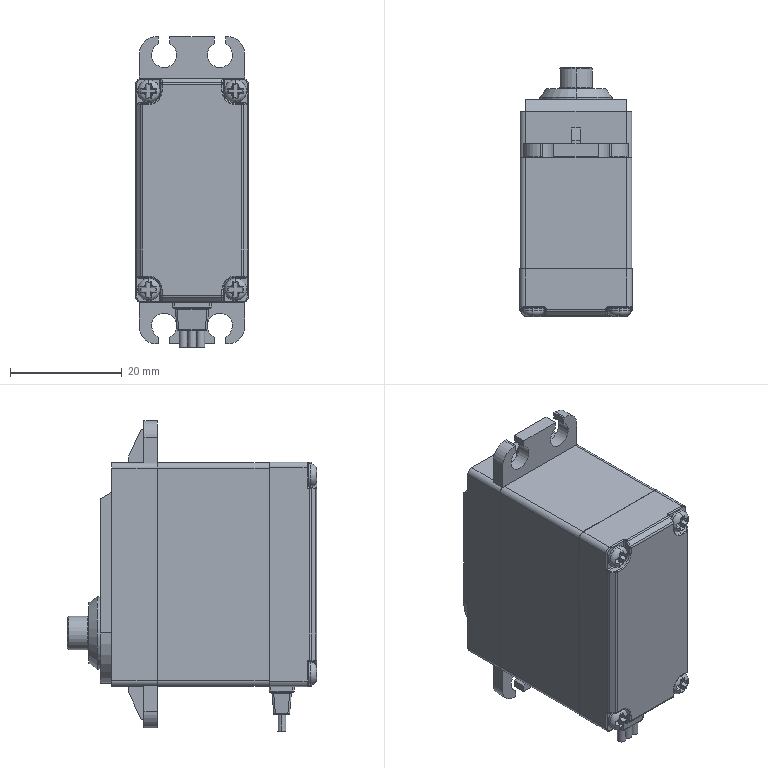Part | SolidWorks | features ICE 27, Fillet 16, Chamfer 2, CombineBodies 2, Extrusion 1, HoleWzd 1, LPattern 1, Revolution 1 | 9 solids | 464 faces | box 20.1 x 44.6 x 55.6 mm | volume 21079 mm3 | plane 188 | cylinder 162 | torus 86 | spline 20 | cone 8 | commonest cylinder face diameters 0.4 x52 2 x36 1 x16 4 x10 0.6 x8 6 x8